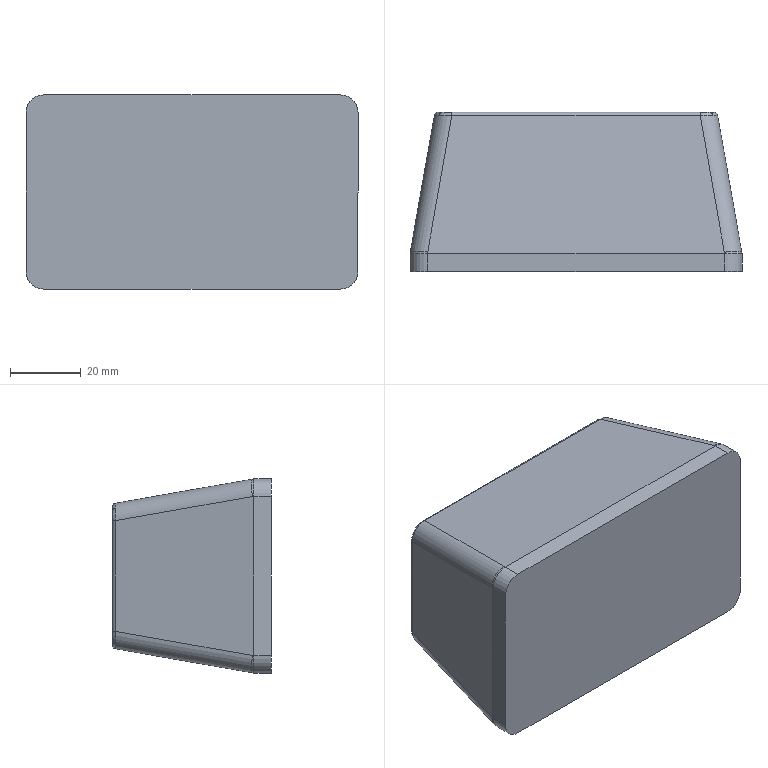Part | SolidWorks | 1 solid | 43 faces | box 94 x 45 x 55 mm | volume 48372 mm3 | cylinder 16 | plane 15 | spline 8 | cone 4 | commonest cylinder face diameters 10 x8 2 x4 7 x4